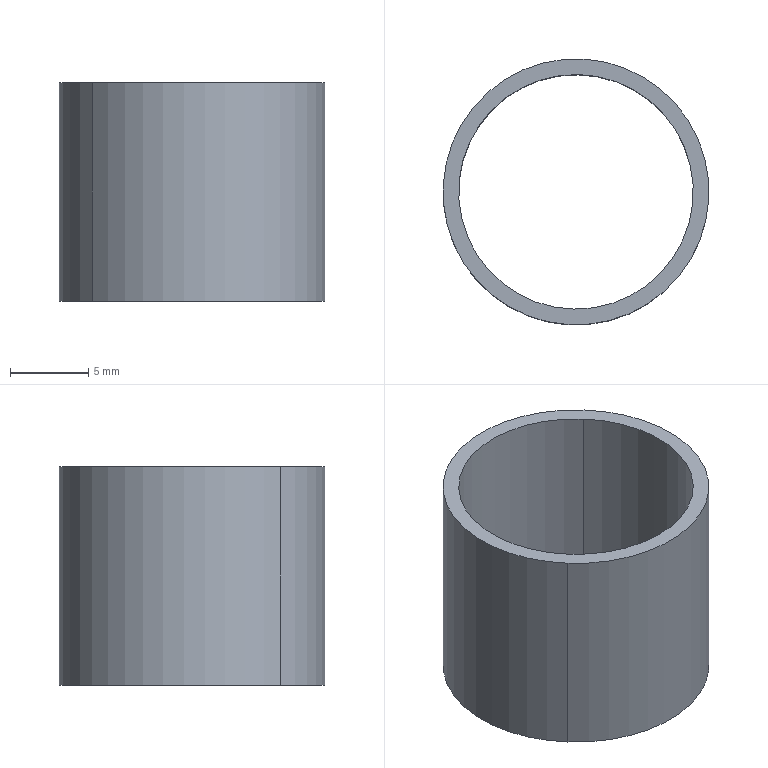Part | SolidWorks | features BaseBody 1 | 1 solid | 6 faces | box 17 x 17 x 14 mm | volume 703.717 mm3 | cylinder 4 | plane 2 | commonest cylinder face diameters 15 x2 17 x2
STEP:
#1=CARTESIAN_POINT('',(228.862,130.136,86.5));
#2=VERTEX_POINT('',#1);
#3=CARTESIAN_POINT('',(216.138,118.864,86.5));
#4=VERTEX_POINT('',#3);
#5=CARTESIAN_POINT('',(222.5,124.5,86.5));
#6=DIRECTION('',(0.,0.,1.));
#7=DIRECTION('',(0.7485,0.6631,0.));
#8=AXIS2_PLACEMENT_3D('',#5,#6,#7);
#9=CIRCLE('',#8,8.5);
#10=EDGE_CURVE('',#2,#4,#9,.T.);
#11=ORIENTED_EDGE('',*,*,#10,.T.);
#12=CARTESIAN_POINT('',(216.138,118.864,100.5));
#13=VERTEX_POINT('',#12);
#14=CARTESIAN_POINT('',(216.138,118.864,102.514));
#15=DIRECTION('',(0.,0.,1.));
#16=VECTOR('',#15,1000.);
#17=LINE('',#14,#16);
#18=EDGE_CURVE('',#4,#13,#17,.T.);
#19=ORIENTED_EDGE('',*,*,#18,.T.);
#20=CARTESIAN_POINT('',(228.862,130.136,100.5));
#21=VERTEX_POINT('',#20);
#22=CARTESIAN_POINT('',(222.5,124.5,100.5));
#23=DIRECTION('',(0.,0.,1.));
#24=DIRECTION('',(0.7485,0.6631,0.));
#25=AXIS2_PLACEMENT_3D('',#22,#23,#24);
#26=CIRCLE('',#25,8.5);
#27=EDGE_CURVE('',#21,#13,#26,.T.);
#28=ORIENTED_EDGE('',*,*,#27,.F.);
#29=CARTESIAN_POINT('',(228.862,130.136,102.514));
#30=DIRECTION('',(0.,0.,1.));
#31=VECTOR('',#30,1000.);
#32=LINE('',#29,#31);
#33=EDGE_CURVE('',#2,#21,#32,.T.);
#34=ORIENTED_EDGE('',*,*,#33,.F.);
#35=EDGE_LOOP('',(#11,#19,#28,#34));
#36=FACE_OUTER_BOUND('',#35,.T.);
#37=CARTESIAN_POINT('',(222.5,124.5,102.514));
#38=DIRECTION('',(0.,0.,1.));
#39=DIRECTION('',(0.7485,0.6631,0.));
#40=AXIS2_PLACEMENT_3D('',#37,#38,#39);
#41=CYLINDRICAL_SURFACE('',#40,8.5);
#42=ADVANCED_FACE('',(#36),#41,.T.);
#43=CARTESIAN_POINT('',(216.886,119.527,86.5));
#44=VERTEX_POINT('',#43);
#45=CARTESIAN_POINT('',(228.114,129.473,86.5));
#46=VERTEX_POINT('',#45);
#47=CARTESIAN_POINT('',(222.5,124.5,86.5));
#48=DIRECTION('',(0.,0.,1.));
#49=DIRECTION('',(0.7485,0.6631,0.));
#50=AXIS2_PLACEMENT_3D('',#47,#48,#49);
#51=CIRCLE('',#50,7.5);
#52=EDGE_CURVE('',#44,#46,#51,.T.);
#53=ORIENTED_EDGE('',*,*,#52,.F.);
#54=CARTESIAN_POINT('',(216.886,119.527,100.5));
#55=VERTEX_POINT('',#54);
#56=CARTESIAN_POINT('',(216.886,119.527,102.514));
#57=DIRECTION('',(0.,0.,1.));
#58=VECTOR('',#57,1000.);
#59=LINE('',#56,#58);
#60=EDGE_CURVE('',#44,#55,#59,.T.);
#61=ORIENTED_EDGE('',*,*,#60,.T.);
#62=CARTESIAN_POINT('',(228.114,129.473,100.5));
#63=VERTEX_POINT('',#62);
#64=CARTESIAN_POINT('',(222.5,124.5,100.5));
#65=DIRECTION('',(0.,0.,1.));
#66=DIRECTION('',(0.7485,0.6631,0.));
#67=AXIS2_PLACEMENT_3D('',#64,#65,#66);
#68=CIRCLE('',#67,7.5);
#69=EDGE_CURVE('',#55,#63,#68,.T.);
#70=ORIENTED_EDGE('',*,*,#69,.T.);
#71=CARTESIAN_POINT('',(228.114,129.473,102.514));
#72=DIRECTION('',(0.,0.,1.));
#73=VECTOR('',#72,1000.);
#74=LINE('',#71,#73);
#75=EDGE_CURVE('',#46,#63,#74,.T.);
#76=ORIENTED_EDGE('',*,*,#75,.F.);
#77=EDGE_LOOP('',(#53,#61,#70,#76));
#78=FACE_OUTER_BOUND('',#77,.T.);
#79=CARTESIAN_POINT('',(222.5,124.5,102.514));
#80=DIRECTION('',(0.,0.,1.));
#81=DIRECTION('',(0.7485,0.6631,0.));
#82=AXIS2_PLACEMENT_3D('',#79,#80,#81);
#83=CYLINDRICAL_SURFACE('',#82,7.5);
#84=ADVANCED_FACE('',(#78),#83,.F.);
#85=ORIENTED_EDGE('',*,*,#60,.F.);
#86=CARTESIAN_POINT('',(222.5,124.5,86.5));
#87=DIRECTION('',(0.,0.,1.));
#88=DIRECTION('',(0.7485,0.6631,0.));
#89=AXIS2_PLACEMENT_3D('',#86,#87,#88);
#90=CIRCLE('',#89,7.5);
#91=EDGE_CURVE('',#46,#44,#90,.T.);
#92=ORIENTED_EDGE('',*,*,#91,.F.);
#93=ORIENTED_EDGE('',*,*,#75,.T.);
#94=CARTESIAN_POINT('',(222.5,124.5,100.5));
#95=DIRECTION('',(0.,0.,1.));
#96=DIRECTION('',(0.7485,0.6631,0.));
#97=AXIS2_PLACEMENT_3D('',#94,#95,#96);
#98=CIRCLE('',#97,7.5);
#99=EDGE_CURVE('',#63,#55,#98,.T.);
#100=ORIENTED_EDGE('',*,*,#99,.T.);
#101=EDGE_LOOP('',(#85,#92,#93,#100));
#102=FACE_OUTER_BOUND('',#101,.T.);
#103=CARTESIAN_POINT('',(222.5,124.5,102.514));
#104=DIRECTION('',(0.,0.,1.));
#105=DIRECTION('',(0.7485,0.6631,0.));
#106=AXIS2_PLACEMENT_3D('',#103,#104,#105);
#107=CYLINDRICAL_SURFACE('',#106,7.5);
#108=ADVANCED_FACE('',(#102),#107,.F.);
#109=ORIENTED_EDGE('',*,*,#10,.F.);
#110=CARTESIAN_POINT('',(222.5,124.5,86.5));
#111=DIRECTION('',(0.,0.,1.));
#112=DIRECTION('',(0.7485,0.6631,0.));
#113=AXIS2_PLACEMENT_3D('',#110,#111,#112);
#114=CIRCLE('',#113,8.5);
#115=EDGE_CURVE('',#4,#2,#114,.T.);
#116=ORIENTED_EDGE('',*,*,#115,.F.);
#117=EDGE_LOOP('',(#109,#116));
#118=FACE_OUTER_BOUND('',#117,.T.);
#119=ORIENTED_EDGE('',*,*,#91,.T.);
#120=ORIENTED_EDGE('',*,*,#52,.T.);
#121=EDGE_LOOP('',(#119,#120));
#122=FACE_BOUND('',#121,.T.);
#123=CARTESIAN_POINT('',(216.864,130.862,86.5));
#124=DIRECTION('',(0.,0.,1.));
#125=DIRECTION('',(0.7485,0.6631,0.));
#126=AXIS2_PLACEMENT_3D('',#123,#124,#125);
#127=PLANE('',#126);
#128=ADVANCED_FACE('',(#118,#122),#127,.F.);
#129=ORIENTED_EDGE('',*,*,#18,.F.);
#130=ORIENTED_EDGE('',*,*,#115,.T.);
#131=ORIENTED_EDGE('',*,*,#33,.T.);
#132=CARTESIAN_POINT('',(222.5,124.5,100.5));
#133=DIRECTION('',(0.,0.,1.));
#134=DIRECTION('',(0.7485,0.6631,0.));
#135=AXIS2_PLACEMENT_3D('',#132,#133,#134);
#136=CIRCLE('',#135,8.5);
#137=EDGE_CURVE('',#13,#21,#136,.T.);
#138=ORIENTED_EDGE('',*,*,#137,.F.);
#139=EDGE_LOOP('',(#129,#130,#131,#138));
#140=FACE_OUTER_BOUND('',#139,.T.);
#141=CARTESIAN_POINT('',(222.5,124.5,102.514));
#142=DIRECTION('',(0.,0.,1.));
#143=DIRECTION('',(0.7485,0.6631,0.));
#144=AXIS2_PLACEMENT_3D('',#141,#142,#143);
#145=CYLINDRICAL_SURFACE('',#144,8.5);
#146=ADVANCED_FACE('',(#140),#145,.T.);
#147=ORIENTED_EDGE('',*,*,#99,.F.);
#148=ORIENTED_EDGE('',*,*,#69,.F.);
#149=EDGE_LOOP('',(#147,#148));
#150=FACE_BOUND('',#149,.T.);
#151=ORIENTED_EDGE('',*,*,#27,.T.);
#152=ORIENTED_EDGE('',*,*,#137,.T.);
#153=EDGE_LOOP('',(#151,#152));
#154=FACE_OUTER_BOUND('',#153,.T.);
#155=CARTESIAN_POINT('',(217.527,130.114,100.5));
#156=DIRECTION('',(0.,0.,-1.));
#157=DIRECTION('',(-0.7485,-0.6631,0.));
#158=AXIS2_PLACEMENT_3D('',#155,#156,#157);
#159=PLANE('',#158);
#160=ADVANCED_FACE('',(#150,#154),#159,.F.);
#161=CLOSED_SHELL('',(#42,#84,#108,#128,#146,#160));
#162=MANIFOLD_SOLID_BREP('',#161);
#163=CARTESIAN_POINT('',(0.,0.,0.));
#164=DIRECTION('',(0.,0.,1.));
#165=DIRECTION('',(1.,0.,0.));
#166=AXIS2_PLACEMENT_3D('',#163,#164,#165);
#167=(LENGTH_UNIT()NAMED_UNIT(*)SI_UNIT(.MILLI.,.METRE.));
#168=UNCERTAINTY_MEASURE_WITH_UNIT(LENGTH_MEASURE(0.00001),#167,'','');
#169=(NAMED_UNIT(*)PLANE_ANGLE_UNIT()SI_UNIT($,.RADIAN.));
#170=(NAMED_UNIT(*)SI_UNIT($,.STERADIAN.)SOLID_ANGLE_UNIT());
#171=(GEOMETRIC_REPRESENTATION_CONTEXT(3)GLOBAL_UNCERTAINTY_ASSIGNED_CONTEXT((#168))GLOBAL_UNIT_ASSIGNED_CONTEXT((#167,#169,#170))REPRESENTATION_CONTEXT('',''));
#172=ADVANCED_BREP_SHAPE_REPRESENTATION('',(#162,#166),#171);